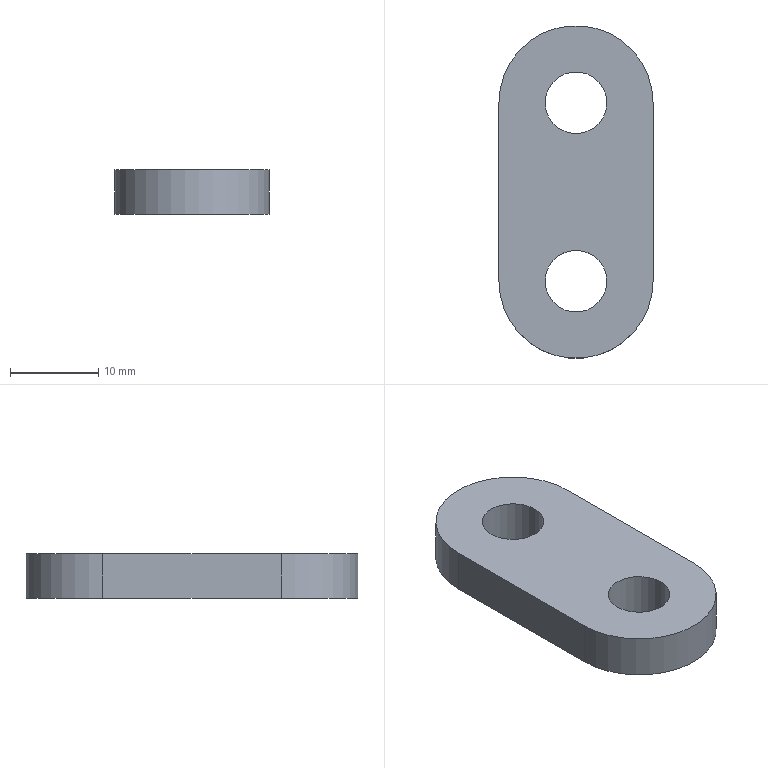Part | SolidWorks | features Extrusion 1 | 1 solid | 10 faces | box 17.5 x 37.76 x 5 mm | volume 2591 mm3 | cylinder 6 | plane 4 | commonest cylinder face diameters 7 x4 17.5 x2
STEP:
#1=CARTESIAN_POINT('',(-3.5,-20.26,5.));
#2=VERTEX_POINT('',#1);
#3=CARTESIAN_POINT('',(3.5,-20.26,5.));
#4=VERTEX_POINT('',#3);
#5=CARTESIAN_POINT('',(0.,-20.26,5.));
#6=DIRECTION('',(0.,0.,1.));
#7=DIRECTION('',(1.,0.,0.));
#8=AXIS2_PLACEMENT_3D('',#5,#6,#7);
#9=CIRCLE('',#8,3.5);
#10=EDGE_CURVE('',#2,#4,#9,.T.);
#11=ORIENTED_EDGE('',*,*,#10,.T.);
#12=CARTESIAN_POINT('',(3.5,-20.26,0.));
#13=VERTEX_POINT('',#12);
#14=CARTESIAN_POINT('',(3.5,-20.26,5.));
#15=DIRECTION('',(0.,0.,-1.));
#16=VECTOR('',#15,1000.);
#17=LINE('',#14,#16);
#18=EDGE_CURVE('',#4,#13,#17,.T.);
#19=ORIENTED_EDGE('',*,*,#18,.T.);
#20=CARTESIAN_POINT('',(-3.5,-20.26,0.));
#21=VERTEX_POINT('',#20);
#22=CARTESIAN_POINT('',(0.,-20.26,0.));
#23=DIRECTION('',(0.,0.,1.));
#24=DIRECTION('',(1.,0.,0.));
#25=AXIS2_PLACEMENT_3D('',#22,#23,#24);
#26=CIRCLE('',#25,3.5);
#27=EDGE_CURVE('',#21,#13,#26,.T.);
#28=ORIENTED_EDGE('',*,*,#27,.F.);
#29=CARTESIAN_POINT('',(-3.5,-20.26,5.));
#30=DIRECTION('',(0.,0.,-1.));
#31=VECTOR('',#30,1000.);
#32=LINE('',#29,#31);
#33=EDGE_CURVE('',#2,#21,#32,.T.);
#34=ORIENTED_EDGE('',*,*,#33,.F.);
#35=EDGE_LOOP('',(#11,#19,#28,#34));
#36=FACE_OUTER_BOUND('',#35,.T.);
#37=CARTESIAN_POINT('',(0.,-20.26,5.));
#38=DIRECTION('',(0.,0.,-1.));
#39=DIRECTION('',(-1.,0.,0.));
#40=AXIS2_PLACEMENT_3D('',#37,#38,#39);
#41=CYLINDRICAL_SURFACE('',#40,3.5);
#42=ADVANCED_FACE('',(#36),#41,.F.);
#43=CARTESIAN_POINT('',(-3.5,0.,5.));
#44=VERTEX_POINT('',#43);
#45=CARTESIAN_POINT('',(3.5,0.,5.));
#46=VERTEX_POINT('',#45);
#47=CARTESIAN_POINT('',(0.,0.,5.));
#48=DIRECTION('',(0.,0.,1.));
#49=DIRECTION('',(1.,0.,0.));
#50=AXIS2_PLACEMENT_3D('',#47,#48,#49);
#51=CIRCLE('',#50,3.5);
#52=EDGE_CURVE('',#44,#46,#51,.T.);
#53=ORIENTED_EDGE('',*,*,#52,.T.);
#54=CARTESIAN_POINT('',(3.5,0.,0.));
#55=VERTEX_POINT('',#54);
#56=CARTESIAN_POINT('',(3.5,0.,5.));
#57=DIRECTION('',(0.,0.,-1.));
#58=VECTOR('',#57,1000.);
#59=LINE('',#56,#58);
#60=EDGE_CURVE('',#46,#55,#59,.T.);
#61=ORIENTED_EDGE('',*,*,#60,.T.);
#62=CARTESIAN_POINT('',(-3.5,0.,0.));
#63=VERTEX_POINT('',#62);
#64=CARTESIAN_POINT('',(0.,0.,0.));
#65=DIRECTION('',(0.,0.,1.));
#66=DIRECTION('',(1.,0.,0.));
#67=AXIS2_PLACEMENT_3D('',#64,#65,#66);
#68=CIRCLE('',#67,3.5);
#69=EDGE_CURVE('',#63,#55,#68,.T.);
#70=ORIENTED_EDGE('',*,*,#69,.F.);
#71=CARTESIAN_POINT('',(-3.5,0.,5.));
#72=DIRECTION('',(0.,0.,-1.));
#73=VECTOR('',#72,1000.);
#74=LINE('',#71,#73);
#75=EDGE_CURVE('',#44,#63,#74,.T.);
#76=ORIENTED_EDGE('',*,*,#75,.F.);
#77=EDGE_LOOP('',(#53,#61,#70,#76));
#78=FACE_OUTER_BOUND('',#77,.T.);
#79=CARTESIAN_POINT('',(0.,0.,5.));
#80=DIRECTION('',(0.,0.,-1.));
#81=DIRECTION('',(-1.,0.,0.));
#82=AXIS2_PLACEMENT_3D('',#79,#80,#81);
#83=CYLINDRICAL_SURFACE('',#82,3.5);
#84=ADVANCED_FACE('',(#78),#83,.F.);
#85=ORIENTED_EDGE('',*,*,#52,.F.);
#86=CARTESIAN_POINT('',(0.,0.,5.));
#87=DIRECTION('',(0.,0.,1.));
#88=DIRECTION('',(1.,0.,0.));
#89=AXIS2_PLACEMENT_3D('',#86,#87,#88);
#90=CIRCLE('',#89,3.5);
#91=EDGE_CURVE('',#46,#44,#90,.T.);
#92=ORIENTED_EDGE('',*,*,#91,.F.);
#93=EDGE_LOOP('',(#85,#92));
#94=FACE_BOUND('',#93,.T.);
#95=CARTESIAN_POINT('',(-8.75,-20.26,5.));
#96=VERTEX_POINT('',#95);
#97=CARTESIAN_POINT('',(8.75,-20.26,5.));
#98=VERTEX_POINT('',#97);
#99=CARTESIAN_POINT('',(0.,-20.26,5.));
#100=DIRECTION('',(0.,0.,1.));
#101=DIRECTION('',(1.,0.,0.));
#102=AXIS2_PLACEMENT_3D('',#99,#100,#101);
#103=CIRCLE('',#102,8.75);
#104=EDGE_CURVE('',#96,#98,#103,.T.);
#105=ORIENTED_EDGE('',*,*,#104,.T.);
#106=CARTESIAN_POINT('',(8.75,0.,5.));
#107=VERTEX_POINT('',#106);
#108=CARTESIAN_POINT('',(8.75,0.,5.));
#109=DIRECTION('',(0.,1.,0.));
#110=VECTOR('',#109,1000.);
#111=LINE('',#108,#110);
#112=EDGE_CURVE('',#98,#107,#111,.T.);
#113=ORIENTED_EDGE('',*,*,#112,.T.);
#114=CARTESIAN_POINT('',(-8.75,0.,5.));
#115=VERTEX_POINT('',#114);
#116=CARTESIAN_POINT('',(0.,0.,5.));
#117=DIRECTION('',(0.,0.,1.));
#118=DIRECTION('',(1.,0.,0.));
#119=AXIS2_PLACEMENT_3D('',#116,#117,#118);
#120=CIRCLE('',#119,8.75);
#121=EDGE_CURVE('',#107,#115,#120,.T.);
#122=ORIENTED_EDGE('',*,*,#121,.T.);
#123=CARTESIAN_POINT('',(-8.75,0.,5.));
#124=DIRECTION('',(0.,-1.,0.));
#125=VECTOR('',#124,1000.);
#126=LINE('',#123,#125);
#127=EDGE_CURVE('',#115,#96,#126,.T.);
#128=ORIENTED_EDGE('',*,*,#127,.T.);
#129=EDGE_LOOP('',(#105,#113,#122,#128));
#130=FACE_OUTER_BOUND('',#129,.T.);
#131=ORIENTED_EDGE('',*,*,#10,.F.);
#132=CARTESIAN_POINT('',(0.,-20.26,5.));
#133=DIRECTION('',(0.,0.,1.));
#134=DIRECTION('',(1.,0.,0.));
#135=AXIS2_PLACEMENT_3D('',#132,#133,#134);
#136=CIRCLE('',#135,3.5);
#137=EDGE_CURVE('',#4,#2,#136,.T.);
#138=ORIENTED_EDGE('',*,*,#137,.F.);
#139=EDGE_LOOP('',(#131,#138));
#140=FACE_BOUND('',#139,.T.);
#141=CARTESIAN_POINT('',(0.,-20.26,5.));
#142=DIRECTION('',(0.,0.,1.));
#143=DIRECTION('',(1.,0.,0.));
#144=AXIS2_PLACEMENT_3D('',#141,#142,#143);
#145=PLANE('',#144);
#146=ADVANCED_FACE('',(#94,#130,#140),#145,.T.);
#147=CARTESIAN_POINT('',(-8.75,-20.26,0.));
#148=VERTEX_POINT('',#147);
#149=CARTESIAN_POINT('',(8.75,-20.26,0.));
#150=VERTEX_POINT('',#149);
#151=CARTESIAN_POINT('',(0.,-20.26,0.));
#152=DIRECTION('',(0.,0.,1.));
#153=DIRECTION('',(1.,0.,0.));
#154=AXIS2_PLACEMENT_3D('',#151,#152,#153);
#155=CIRCLE('',#154,8.75);
#156=EDGE_CURVE('',#148,#150,#155,.T.);
#157=ORIENTED_EDGE('',*,*,#156,.F.);
#158=CARTESIAN_POINT('',(-8.75,0.,0.));
#159=VERTEX_POINT('',#158);
#160=CARTESIAN_POINT('',(-8.75,0.,0.));
#161=DIRECTION('',(0.,-1.,0.));
#162=VECTOR('',#161,1000.);
#163=LINE('',#160,#162);
#164=EDGE_CURVE('',#159,#148,#163,.T.);
#165=ORIENTED_EDGE('',*,*,#164,.F.);
#166=CARTESIAN_POINT('',(8.75,0.,0.));
#167=VERTEX_POINT('',#166);
#168=CARTESIAN_POINT('',(0.,0.,0.));
#169=DIRECTION('',(0.,0.,1.));
#170=DIRECTION('',(1.,0.,0.));
#171=AXIS2_PLACEMENT_3D('',#168,#169,#170);
#172=CIRCLE('',#171,8.75);
#173=EDGE_CURVE('',#167,#159,#172,.T.);
#174=ORIENTED_EDGE('',*,*,#173,.F.);
#175=CARTESIAN_POINT('',(8.75,0.,0.));
#176=DIRECTION('',(0.,1.,0.));
#177=VECTOR('',#176,1000.);
#178=LINE('',#175,#177);
#179=EDGE_CURVE('',#150,#167,#178,.T.);
#180=ORIENTED_EDGE('',*,*,#179,.F.);
#181=EDGE_LOOP('',(#157,#165,#174,#180));
#182=FACE_OUTER_BOUND('',#181,.T.);
#183=ORIENTED_EDGE('',*,*,#69,.T.);
#184=CARTESIAN_POINT('',(0.,0.,0.));
#185=DIRECTION('',(0.,0.,1.));
#186=DIRECTION('',(1.,0.,0.));
#187=AXIS2_PLACEMENT_3D('',#184,#185,#186);
#188=CIRCLE('',#187,3.5);
#189=EDGE_CURVE('',#55,#63,#188,.T.);
#190=ORIENTED_EDGE('',*,*,#189,.T.);
#191=EDGE_LOOP('',(#183,#190));
#192=FACE_BOUND('',#191,.T.);
#193=ORIENTED_EDGE('',*,*,#27,.T.);
#194=CARTESIAN_POINT('',(0.,-20.26,0.));
#195=DIRECTION('',(0.,0.,1.));
#196=DIRECTION('',(1.,0.,0.));
#197=AXIS2_PLACEMENT_3D('',#194,#195,#196);
#198=CIRCLE('',#197,3.5);
#199=EDGE_CURVE('',#13,#21,#198,.T.);
#200=ORIENTED_EDGE('',*,*,#199,.T.);
#201=EDGE_LOOP('',(#193,#200));
#202=FACE_BOUND('',#201,.T.);
#203=CARTESIAN_POINT('',(0.,-20.26,0.));
#204=DIRECTION('',(0.,0.,1.));
#205=DIRECTION('',(1.,0.,0.));
#206=AXIS2_PLACEMENT_3D('',#203,#204,#205);
#207=PLANE('',#206);
#208=ADVANCED_FACE('',(#182,#192,#202),#207,.F.);
#209=ORIENTED_EDGE('',*,*,#156,.T.);
#210=CARTESIAN_POINT('',(8.75,-20.26,5.));
#211=DIRECTION('',(0.,0.,-1.));
#212=VECTOR('',#211,1000.);
#213=LINE('',#210,#212);
#214=EDGE_CURVE('',#98,#150,#213,.T.);
#215=ORIENTED_EDGE('',*,*,#214,.F.);
#216=ORIENTED_EDGE('',*,*,#104,.F.);
#217=CARTESIAN_POINT('',(-8.75,-20.26,5.));
#218=DIRECTION('',(0.,0.,-1.));
#219=VECTOR('',#218,1000.);
#220=LINE('',#217,#219);
#221=EDGE_CURVE('',#96,#148,#220,.T.);
#222=ORIENTED_EDGE('',*,*,#221,.T.);
#223=EDGE_LOOP('',(#209,#215,#216,#222));
#224=FACE_OUTER_BOUND('',#223,.T.);
#225=CARTESIAN_POINT('',(0.,-20.26,5.));
#226=DIRECTION('',(0.,0.,-1.));
#227=DIRECTION('',(-1.,0.,0.));
#228=AXIS2_PLACEMENT_3D('',#225,#226,#227);
#229=CYLINDRICAL_SURFACE('',#228,8.75);
#230=ADVANCED_FACE('',(#224),#229,.T.);
#231=ORIENTED_EDGE('',*,*,#179,.T.);
#232=CARTESIAN_POINT('',(8.75,0.,5.));
#233=DIRECTION('',(0.,0.,-1.));
#234=VECTOR('',#233,1000.);
#235=LINE('',#232,#234);
#236=EDGE_CURVE('',#107,#167,#235,.T.);
#237=ORIENTED_EDGE('',*,*,#236,.F.);
#238=ORIENTED_EDGE('',*,*,#112,.F.);
#239=ORIENTED_EDGE('',*,*,#214,.T.);
#240=EDGE_LOOP('',(#231,#237,#238,#239));
#241=FACE_OUTER_BOUND('',#240,.T.);
#242=CARTESIAN_POINT('',(8.75,0.,5.));
#243=DIRECTION('',(-1.,0.,0.));
#244=DIRECTION('',(0.,0.,1.));
#245=AXIS2_PLACEMENT_3D('',#242,#243,#244);
#246=PLANE('',#245);
#247=ADVANCED_FACE('',(#241),#246,.F.);
#248=ORIENTED_EDGE('',*,*,#173,.T.);
#249=CARTESIAN_POINT('',(-8.75,0.,5.));
#250=DIRECTION('',(0.,0.,-1.));
#251=VECTOR('',#250,1000.);
#252=LINE('',#249,#251);
#253=EDGE_CURVE('',#115,#159,#252,.T.);
#254=ORIENTED_EDGE('',*,*,#253,.F.);
#255=ORIENTED_EDGE('',*,*,#121,.F.);
#256=ORIENTED_EDGE('',*,*,#236,.T.);
#257=EDGE_LOOP('',(#248,#254,#255,#256));
#258=FACE_OUTER_BOUND('',#257,.T.);
#259=CARTESIAN_POINT('',(0.,0.,5.));
#260=DIRECTION('',(0.,0.,-1.));
#261=DIRECTION('',(-1.,0.,0.));
#262=AXIS2_PLACEMENT_3D('',#259,#260,#261);
#263=CYLINDRICAL_SURFACE('',#262,8.75);
#264=ADVANCED_FACE('',(#258),#263,.T.);
#265=ORIENTED_EDGE('',*,*,#164,.T.);
#266=ORIENTED_EDGE('',*,*,#221,.F.);
#267=ORIENTED_EDGE('',*,*,#127,.F.);
#268=ORIENTED_EDGE('',*,*,#253,.T.);
#269=EDGE_LOOP('',(#265,#266,#267,#268));
#270=FACE_OUTER_BOUND('',#269,.T.);
#271=CARTESIAN_POINT('',(-8.75,0.,5.));
#272=DIRECTION('',(1.,0.,0.));
#273=DIRECTION('',(0.,0.,-1.));
#274=AXIS2_PLACEMENT_3D('',#271,#272,#273);
#275=PLANE('',#274);
#276=ADVANCED_FACE('',(#270),#275,.F.);
#277=ORIENTED_EDGE('',*,*,#60,.F.);
#278=ORIENTED_EDGE('',*,*,#91,.T.);
#279=ORIENTED_EDGE('',*,*,#75,.T.);
#280=ORIENTED_EDGE('',*,*,#189,.F.);
#281=EDGE_LOOP('',(#277,#278,#279,#280));
#282=FACE_OUTER_BOUND('',#281,.T.);
#283=CARTESIAN_POINT('',(0.,0.,5.));
#284=DIRECTION('',(0.,0.,-1.));
#285=DIRECTION('',(-1.,0.,0.));
#286=AXIS2_PLACEMENT_3D('',#283,#284,#285);
#287=CYLINDRICAL_SURFACE('',#286,3.5);
#288=ADVANCED_FACE('',(#282),#287,.F.);
#289=ORIENTED_EDGE('',*,*,#18,.F.);
#290=ORIENTED_EDGE('',*,*,#137,.T.);
#291=ORIENTED_EDGE('',*,*,#33,.T.);
#292=ORIENTED_EDGE('',*,*,#199,.F.);
#293=EDGE_LOOP('',(#289,#290,#291,#292));
#294=FACE_OUTER_BOUND('',#293,.T.);
#295=CARTESIAN_POINT('',(0.,-20.26,5.));
#296=DIRECTION('',(0.,0.,-1.));
#297=DIRECTION('',(-1.,0.,0.));
#298=AXIS2_PLACEMENT_3D('',#295,#296,#297);
#299=CYLINDRICAL_SURFACE('',#298,3.5);
#300=ADVANCED_FACE('',(#294),#299,.F.);
#301=CLOSED_SHELL('',(#42,#84,#146,#208,#230,#247,#264,#276,#288,#300));
#302=MANIFOLD_SOLID_BREP('',#301);
#303=CARTESIAN_POINT('',(0.,0.,0.));
#304=DIRECTION('',(0.,0.,1.));
#305=DIRECTION('',(1.,0.,0.));
#306=AXIS2_PLACEMENT_3D('',#303,#304,#305);
#307=(LENGTH_UNIT()NAMED_UNIT(*)SI_UNIT(.MILLI.,.METRE.));
#308=UNCERTAINTY_MEASURE_WITH_UNIT(LENGTH_MEASURE(0.00001),#307,'','');
#309=(NAMED_UNIT(*)PLANE_ANGLE_UNIT()SI_UNIT($,.RADIAN.));
#310=(NAMED_UNIT(*)SI_UNIT($,.STERADIAN.)SOLID_ANGLE_UNIT());
#311=(GEOMETRIC_REPRESENTATION_CONTEXT(3)GLOBAL_UNCERTAINTY_ASSIGNED_CONTEXT((#308))GLOBAL_UNIT_ASSIGNED_CONTEXT((#307,#309,#310))REPRESENTATION_CONTEXT('',''));
#312=ADVANCED_BREP_SHAPE_REPRESENTATION('',(#302,#306),#311);